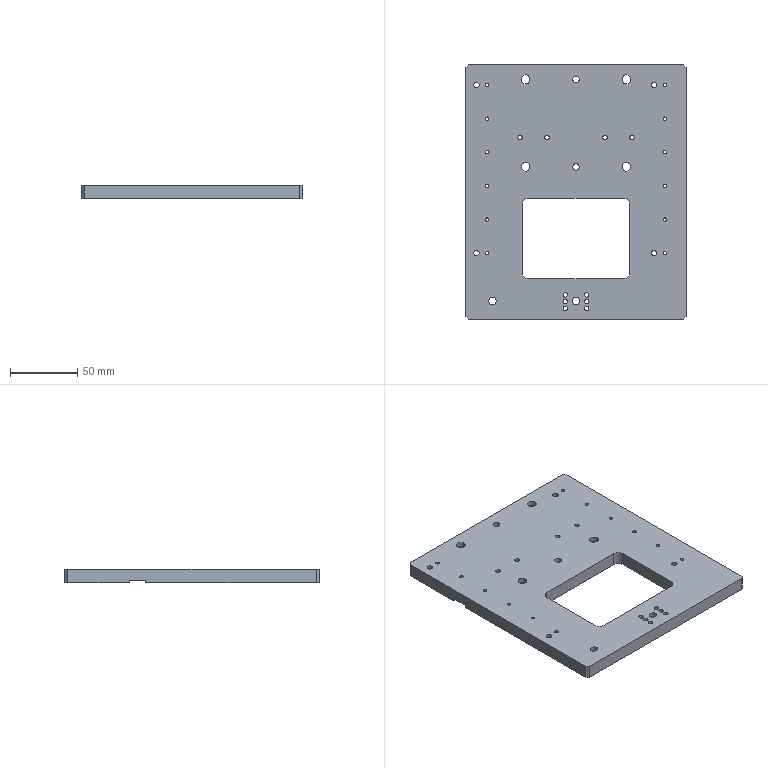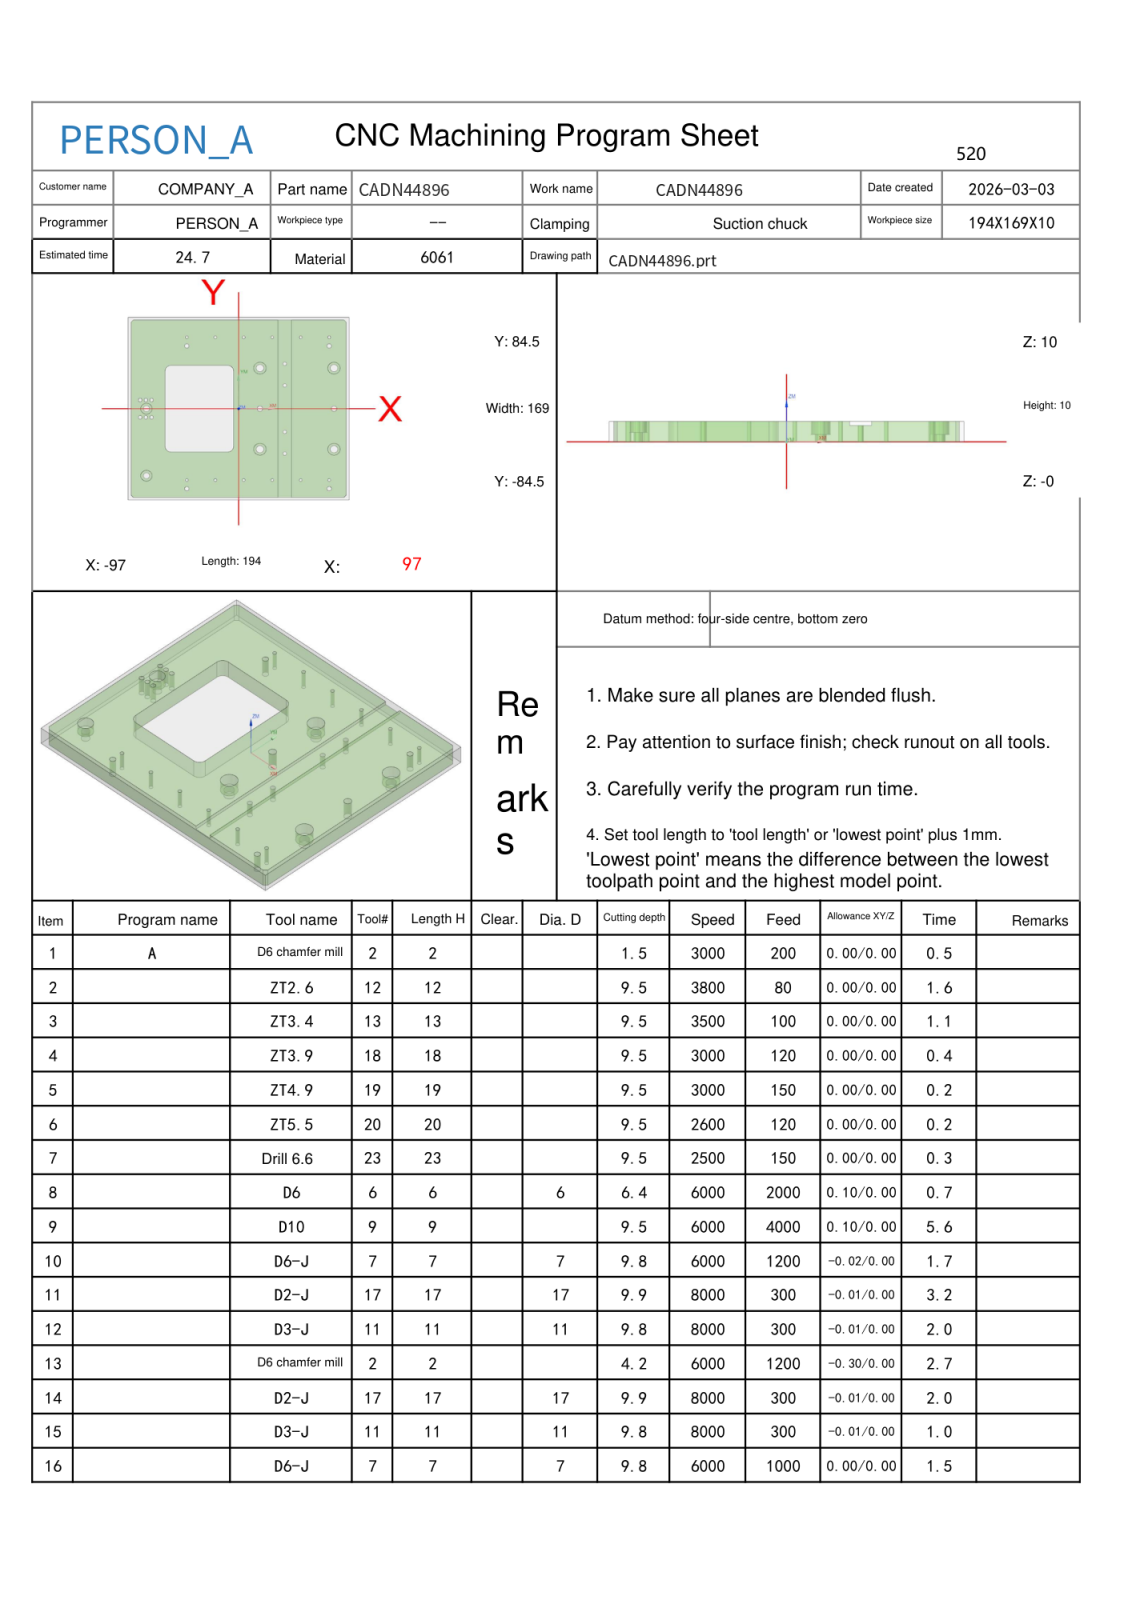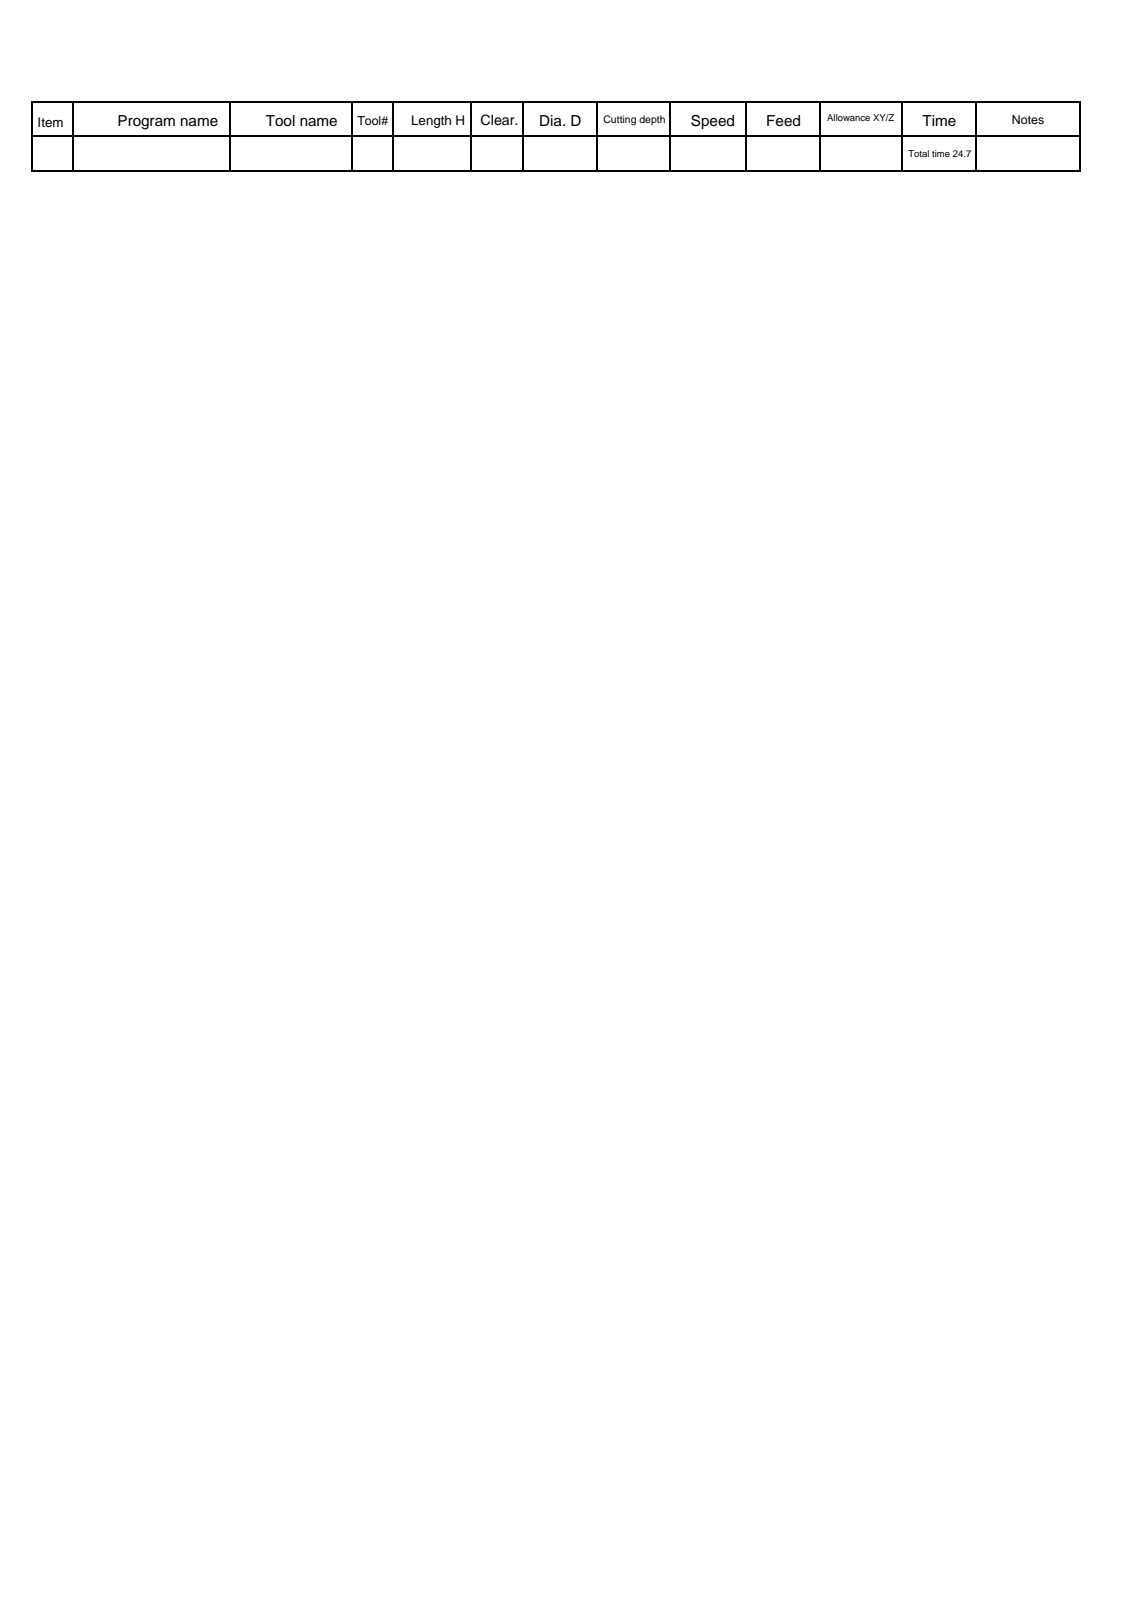NC program | NX | posted by the shop | part box 164 x 189 x 10 mm
Lines 2444 to 4061 of 4061, first 1295 of 1618 lines:
N12 T11 M06
(D3-J  D=3. R=0. H=11 ce=-0.01 di=0.00)
(D.N=11 MAX_Z=40. MIN_Z=0.15 Time=2.03M)
G00 G90 G54 X-81.065 Y1.225 M03 S8000
G43 H11 Z40.
M08
Z5.1
G01 X-81.111 Z5.098 F300.
X-81.384 Y1.169 Z5.083
X-81.637 Y1.053 Z5.068
X-81.857 Y.882 Z5.054
X-82.034 Y.667 Z5.039
X-82.157 Y.417 Z5.025
X-82.221 Y.146 Z5.01
X-82.225 Y-.111 Z4.997
X-82.167 Y-.389 Z4.982
X-82.046 Y-.647 Z4.967
X-81.87 Y-.87 Z4.952
X-81.647 Y-1.046 Z4.937
X-81.389 Y-1.167 Z4.922
X-81.111 Y-1.225 Z4.907
X-80.889 Z4.896
X-80.611 Y-1.167 Z4.881
X-80.353 Y-1.046 Z4.866
X-80.13 Y-.87 Z4.851
X-79.954 Y-.647 Z4.836
X-79.833 Y-.389 Z4.821
X-79.775 Y-.111 Z4.806
Y.111 Z4.794
X-79.833 Y.389 Z4.78
X-79.954 Y.647 Z4.765
X-80.13 Y.87 Z4.75
X-80.353 Y1.046 Z4.735
X-80.611 Y1.167 Z4.72
X-80.889 Y1.225 Z4.705
X-81.111 Z4.693
X-81.384 Y1.169 Z4.679
X-81.637 Y1.053 Z4.664
X-81.857 Y.882 Z4.65
X-82.034 Y.667 Z4.635
X-82.157 Y.417 Z4.62
X-82.221 Y.146 Z4.606
X-82.225 Y.035 Z4.6
G41 D11
X-82.26 Y0.0
G03 X-81. Y-1.26 Z4.476 I1.26 J0.0
X-79.74 Y0.0 Z4.353 I0.0 J1.26
X-81. Y1.26 Z4.229 I-1.26 J0.0
X-82.26 Y0.0 Z4.106 I0.0 J-1.26
X-81. Y-1.26 Z3.982 I1.26 J0.0
X-79.74 Y0.0 Z3.858 I0.0 J1.26
X-81. Y1.26 Z3.735 I-1.26 J0.0
X-82.26 Y0.0 Z3.611 I0.0 J-1.26
X-81. Y-1.26 Z3.488 I1.26 J0.0
X-79.74 Y0.0 Z3.364 I0.0 J1.26
X-81. Y1.26 Z3.24 I-1.26 J0.0
X-82.26 Y0.0 Z3.117 I0.0 J-1.26
X-81. Y-1.26 Z2.993 I1.26 J0.0
X-79.74 Y0.0 Z2.869 I0.0 J1.26
X-81. Y1.26 Z2.746 I-1.26 J0.0
X-82.26 Y0.0 Z2.622 I0.0 J-1.26
X-81. Y-1.26 Z2.499 I1.26 J0.0
X-79.74 Y0.0 Z2.375 I0.0 J1.26
X-81. Y1.26 Z2.251 I-1.26 J0.0
X-82.26 Y0.0 Z2.128 I0.0 J-1.26
X-81. Y-1.26 Z2.004 I1.26 J0.0
X-79.74 Y0.0 Z1.881 I0.0 J1.26
X-81. Y1.26 Z1.757 I-1.26 J0.0
X-82.26 Y0.0 Z1.633 I0.0 J-1.26
X-81. Y-1.26 Z1.51 I1.26 J0.0
X-79.74 Y0.0 Z1.386 I0.0 J1.26
X-81. Y1.26 Z1.263 I-1.26 J0.0
X-82.26 Y0.0 Z1.139 I0.0 J-1.26
X-81. Y-1.26 Z1.015 I1.26 J0.0
X-79.74 Y0.0 Z.892 I0.0 J1.26
X-81. Y1.26 Z.768 I-1.26 J0.0
X-82.26 Y0.0 Z.644 I0.0 J-1.26
X-81. Y-1.26 Z.521 I1.26 J0.0
X-79.74 Y0.0 Z.397 I0.0 J1.26
X-81. Y1.26 Z.274 I-1.26 J0.0
X-82.26 Y0.0 Z.15 I0.0 J-1.26
X-81. Y-1.26 I1.26 J0.0
X-79.74 Y0.0 I0.0 J1.26
X-81. Y1.26 I-1.26 J0.0
X-82.26 Y0.0 I0.0 J-1.26
X-82.197 Y-.393 I1.26 J0.0
G01 X-82.186 Y-.419
X-82.161 Y-.432
X-82.134 Y-.425
G40 X-82.086 Y-.41
Z1.15
G00 Z40.
X-81.065 Y-60.775
Z5.1
G01 X-81.111 Z5.098
X-81.384 Y-60.831 Z5.083
X-81.637 Y-60.947 Z5.068
X-81.857 Y-61.118 Z5.054
X-82.034 Y-61.333 Z5.039
X-82.157 Y-61.583 Z5.025
X-82.221 Y-61.854 Z5.01
X-82.225 Y-62.111 Z4.997
X-82.167 Y-62.389 Z4.982
X-82.046 Y-62.647 Z4.967
X-81.87 Y-62.87 Z4.952
X-81.647 Y-63.046 Z4.937
X-81.389 Y-63.167 Z4.922
X-81.111 Y-63.225 Z4.907
X-80.889 Z4.896
X-80.611 Y-63.167 Z4.881
X-80.353 Y-63.046 Z4.866
X-80.13 Y-62.87 Z4.851
X-79.954 Y-62.647 Z4.836
X-79.833 Y-62.389 Z4.821
X-79.775 Y-62.111 Z4.806
Y-61.889 Z4.794
X-79.833 Y-61.611 Z4.78
X-79.954 Y-61.353 Z4.765
X-80.13 Y-61.13 Z4.75
X-80.353 Y-60.954 Z4.735
X-80.611 Y-60.833 Z4.72
X-80.889 Y-60.775 Z4.705
X-81.111 Z4.693
X-81.384 Y-60.831 Z4.679
X-81.637 Y-60.947 Z4.664
X-81.857 Y-61.118 Z4.65
X-82.034 Y-61.333 Z4.635
X-82.157 Y-61.583 Z4.62
X-82.221 Y-61.854 Z4.606
X-82.225 Y-61.965 Z4.6
G41 D11
X-82.26 Y-62.
G03 X-81. Y-63.26 Z4.476 I1.26 J0.0
X-79.74 Y-62. Z4.353 I0.0 J1.26
X-81. Y-60.74 Z4.229 I-1.26 J0.0
X-82.26 Y-62. Z4.106 I0.0 J-1.26
X-81. Y-63.26 Z3.982 I1.26 J0.0
X-79.74 Y-62. Z3.858 I0.0 J1.26
X-81. Y-60.74 Z3.735 I-1.26 J0.0
X-82.26 Y-62. Z3.611 I0.0 J-1.26
X-81. Y-63.26 Z3.488 I1.26 J0.0
X-79.74 Y-62. Z3.364 I0.0 J1.26
X-81. Y-60.74 Z3.24 I-1.26 J0.0
X-82.26 Y-62. Z3.117 I0.0 J-1.26
X-81. Y-63.26 Z2.993 I1.26 J0.0
X-79.74 Y-62. Z2.869 I0.0 J1.26
X-81. Y-60.74 Z2.746 I-1.26 J0.0
X-82.26 Y-62. Z2.622 I0.0 J-1.26
X-81. Y-63.26 Z2.499 I1.26 J0.0
X-79.74 Y-62. Z2.375 I0.0 J1.26
X-81. Y-60.74 Z2.251 I-1.26 J0.0
X-82.26 Y-62. Z2.128 I0.0 J-1.26
X-81. Y-63.26 Z2.004 I1.26 J0.0
X-79.74 Y-62. Z1.881 I0.0 J1.26
X-81. Y-60.74 Z1.757 I-1.26 J0.0
X-82.26 Y-62. Z1.633 I0.0 J-1.26
X-81. Y-63.26 Z1.51 I1.26 J0.0
X-79.74 Y-62. Z1.386 I0.0 J1.26
X-81. Y-60.74 Z1.263 I-1.26 J0.0
X-82.26 Y-62. Z1.139 I0.0 J-1.26
X-81. Y-63.26 Z1.015 I1.26 J0.0
X-79.74 Y-62. Z.892 I0.0 J1.26
X-81. Y-60.74 Z.768 I-1.26 J0.0
X-82.26 Y-62. Z.644 I0.0 J-1.26
X-81. Y-63.26 Z.521 I1.26 J0.0
X-79.74 Y-62. Z.397 I0.0 J1.26
X-81. Y-60.74 Z.274 I-1.26 J0.0
X-82.26 Y-62. Z.15 I0.0 J-1.26
X-81. Y-63.26 I1.26 J0.0
X-79.74 Y-62. I0.0 J1.26
X-81. Y-60.74 I-1.26 J0.0
X-82.26 Y-62. I0.0 J-1.26
X-82.197 Y-62.393 I1.26 J0.0
G01 X-82.186 Y-62.419
X-82.161 Y-62.432
X-82.134 Y-62.425
G40 X-82.086 Y-62.41
Z1.15
G00 Z40.
X20.087 Y-38.613
Z4.1
G01 X20.278 Y-38.323 Z4.082
X20.412 Y-37.988 Z4.063
X20.475 Y-37.633 Z4.044
Y-37.367 Z4.03
X20.412 Y-37.012 Z4.011
X20.278 Y-36.677 Z3.992
X20.08 Y-36.375 Z3.973
X19.825 Y-36.12 Z3.954
X19.523 Y-35.922 Z3.936
X19.188 Y-35.788 Z3.917
X18.833 Y-35.725 Z3.898
X18.567 Z3.884
X18.212 Y-35.788 Z3.865
X17.877 Y-35.922 Z3.846
X17.575 Y-36.12 Z3.827
X17.32 Y-36.375 Z3.808
X17.122 Y-36.677 Z3.789
X16.988 Y-37.012 Z3.77
X16.925 Y-37.367 Z3.751
Y-37.633 Z3.737
X16.987 Y-37.984 Z3.719
X17.117 Y-38.314 Z3.7
X17.311 Y-38.613 Z3.682
X17.56 Y-38.867 Z3.663
X17.854 Y-39.066 Z3.644
X18.182 Y-39.203 Z3.626
X18.531 Y-39.272 Z3.607
X18.665 Y-39.275 Z3.6
G41 D11
X18.7 Y-39.31
G03 X20.51 Y-37.5 Z3.477 I0.0 J1.81
X18.7 Y-35.69 Z3.354 I-1.81 J0.0
X16.89 Y-37.5 Z3.23 I0.0 J-1.81
X18.7 Y-39.31 Z3.107 I1.81 J0.0
X20.51 Y-37.5 Z2.984 I0.0 J1.81
X18.7 Y-35.69 Z2.861 I-1.81 J0.0
X16.89 Y-37.5 Z2.738 I0.0 J-1.81
X18.7 Y-39.31 Z2.614 I1.81 J0.0
X20.51 Y-37.5 Z2.491 I0.0 J1.81
X18.7 Y-35.69 Z2.368 I-1.81 J0.0
X16.89 Y-37.5 Z2.245 I0.0 J-1.81
X18.7 Y-39.31 Z2.121 I1.81 J0.0
X20.51 Y-37.5 Z1.998 I0.0 J1.81
X18.7 Y-35.69 Z1.875 I-1.81 J0.0
X16.89 Y-37.5 Z1.752 I0.0 J-1.81
X18.7 Y-39.31 Z1.629 I1.81 J0.0
X20.51 Y-37.5 Z1.505 I0.0 J1.81
X18.7 Y-35.69 Z1.382 I-1.81 J0.0
X16.89 Y-37.5 Z1.259 I0.0 J-1.81
X18.7 Y-39.31 Z1.136 I1.81 J0.0
X20.51 Y-37.5 Z1.013 I0.0 J1.81
X18.7 Y-35.69 Z.889 I-1.81 J0.0
X16.89 Y-37.5 Z.766 I0.0 J-1.81
X18.7 Y-39.31 Z.643 I1.81 J0.0
X20.51 Y-37.5 Z.52 I0.0 J1.81
X18.7 Y-35.69 Z.396 I-1.81 J0.0
X16.89 Y-37.5 Z.273 I0.0 J-1.81
X18.7 Y-39.31 Z.15 I1.81 J0.0
X20.51 Y-37.5 I0.0 J1.81
X18.7 Y-35.69 I-1.81 J0.0
X16.89 Y-37.5 I0.0 J-1.81
X18.7 Y-39.31 I1.81 J0.0
X19.097 Y-39.266 I0.0 J1.81
G01 X19.123 Y-39.258
X19.138 Y-39.234
X19.135 Y-39.206
G40 X19.124 Y-39.157
Z1.15
G00 Z40.
X84.813 Y-36.112
Z4.1
G01 X84.523 Y-35.922 Z4.082
X84.188 Y-35.788 Z4.063
X83.833 Y-35.725 Z4.044
X83.567 Z4.03
X83.212 Y-35.788 Z4.011
X82.877 Y-35.922 Z3.992
X82.575 Y-36.12 Z3.973
X82.32 Y-36.375 Z3.954
X82.122 Y-36.677 Z3.936
X81.988 Y-37.012 Z3.917
X81.925 Y-37.367 Z3.898
Y-37.633 Z3.884
X81.963 Y-37.889 Z3.87
X82.037 Y-38.136 Z3.857
X82.147 Y-38.369 Z3.843
X82.294 Y-38.592 Z3.829
X82.551 Y-38.86 Z3.81
X82.858 Y-39.068 Z3.79
X83.201 Y-39.209 Z3.771
X83.567 Y-39.275 Z3.751
X83.833 Z3.737
X84.184 Y-39.213 Z3.719
X84.514 Y-39.083 Z3.7
X84.813 Y-38.889 Z3.682
X85.067 Y-38.64 Z3.663
X85.266 Y-38.346 Z3.644
X85.403 Y-38.018 Z3.626
X85.472 Y-37.669 Z3.607
X85.475 Y-37.535 Z3.6
G41 D11
X85.51 Y-37.5
G03 X83.7 Y-35.69 Z3.477 I-1.81 J0.0
X81.89 Y-37.5 Z3.354 I0.0 J-1.81
X82.191 Y-38.5 Z3.308 I1.81 J0.0
X83.7 Y-39.31 Z3.23 I1.509 J1.
X85.51 Y-37.5 Z3.107 I0.0 J1.81
X83.7 Y-35.69 Z2.984 I-1.81 J0.0
X81.89 Y-37.5 Z2.861 I0.0 J-1.81
X82.191 Y-38.5 Z2.815 I1.81 J0.0
X83.7 Y-39.31 Z2.738 I1.509 J1.
X85.51 Y-37.5 Z2.614 I0.0 J1.81
X83.7 Y-35.69 Z2.491 I-1.81 J0.0
X81.89 Y-37.5 Z2.368 I0.0 J-1.81
X82.191 Y-38.5 Z2.322 I1.81 J0.0
X83.7 Y-39.31 Z2.245 I1.509 J1.
X85.51 Y-37.5 Z2.121 I0.0 J1.81
X83.7 Y-35.69 Z1.998 I-1.81 J0.0
X81.89 Y-37.5 Z1.875 I0.0 J-1.81
X82.191 Y-38.5 Z1.829 I1.81 J0.0
X83.7 Y-39.31 Z1.752 I1.509 J1.
X85.51 Y-37.5 Z1.629 I0.0 J1.81
X83.7 Y-35.69 Z1.505 I-1.81 J0.0
X81.89 Y-37.5 Z1.382 I0.0 J-1.81
X82.191 Y-38.5 Z1.336 I1.81 J0.0
X83.7 Y-39.31 Z1.259 I1.509 J1.
X85.51 Y-37.5 Z1.136 I0.0 J1.81
X83.7 Y-35.69 Z1.013 I-1.81 J0.0
X81.89 Y-37.5 Z.889 I0.0 J-1.81
X82.191 Y-38.5 Z.843 I1.81 J0.0
X83.7 Y-39.31 Z.766 I1.509 J1.
X85.51 Y-37.5 Z.643 I0.0 J1.81
X83.7 Y-35.69 Z.52 I-1.81 J0.0
X81.89 Y-37.5 Z.396 I0.0 J-1.81
X82.191 Y-38.5 Z.351 I1.81 J0.0
X83.7 Y-39.31 Z.273 I1.509 J1.
X85.51 Y-37.5 Z.15 I0.0 J1.81
X83.7 Y-35.69 I-1.81 J0.0
X81.89 Y-37.5 I0.0 J-1.81
X83.7 Y-39.31 I1.81 J0.0
X85.51 Y-37.5 I0.0 J1.81
X85.466 Y-37.103 I-1.81 J0.0
G01 X85.458 Y-37.077
X85.434 Y-37.062
X85.406 Y-37.065
G40 X85.357 Y-37.076
Z1.15
G00 Z40.
X84.813 Y38.888
Z4.1
G01 X84.523 Y39.078 Z4.082
X84.188 Y39.212 Z4.063
X83.833 Y39.275 Z4.044
X83.567 Z4.03
X83.212 Y39.212 Z4.011
X82.877 Y39.078 Z3.992
X82.575 Y38.88 Z3.973
X82.32 Y38.625 Z3.954
X82.122 Y38.323 Z3.936
X81.988 Y37.988 Z3.917
X81.925 Y37.633 Z3.898
Y37.367 Z3.884
X81.963 Y37.111 Z3.87
X82.037 Y36.864 Z3.857
X82.147 Y36.631 Z3.843
X82.294 Y36.408 Z3.829
X82.551 Y36.14 Z3.81
X82.858 Y35.932 Z3.79
X83.201 Y35.791 Z3.771
X83.567 Y35.725 Z3.751
X83.833 Z3.737
X84.184 Y35.787 Z3.719
X84.514 Y35.917 Z3.7
X84.813 Y36.111 Z3.682
X85.067 Y36.36 Z3.663
X85.266 Y36.654 Z3.644
X85.403 Y36.982 Z3.626
X85.472 Y37.331 Z3.607
X85.475 Y37.465 Z3.6
G41 D11
X85.51 Y37.5
G03 X83.7 Y39.31 Z3.477 I-1.81 J0.0
X81.89 Y37.5 Z3.354 I0.0 J-1.81
X82.191 Y36.5 Z3.308 I1.81 J0.0
X83.7 Y35.69 Z3.23 I1.509 J1.
X85.51 Y37.5 Z3.107 I0.0 J1.81
X83.7 Y39.31 Z2.984 I-1.81 J0.0
X81.89 Y37.5 Z2.861 I0.0 J-1.81
X82.191 Y36.5 Z2.815 I1.81 J0.0
X83.7 Y35.69 Z2.738 I1.509 J1.
X85.51 Y37.5 Z2.614 I0.0 J1.81
X83.7 Y39.31 Z2.491 I-1.81 J0.0
X81.89 Y37.5 Z2.368 I0.0 J-1.81
X82.191 Y36.5 Z2.322 I1.81 J0.0
X83.7 Y35.69 Z2.245 I1.509 J1.
X85.51 Y37.5 Z2.121 I0.0 J1.81
X83.7 Y39.31 Z1.998 I-1.81 J0.0
X81.89 Y37.5 Z1.875 I0.0 J-1.81
X82.191 Y36.5 Z1.829 I1.81 J0.0
X83.7 Y35.69 Z1.752 I1.509 J1.
X85.51 Y37.5 Z1.629 I0.0 J1.81
X83.7 Y39.31 Z1.505 I-1.81 J0.0
X81.89 Y37.5 Z1.382 I0.0 J-1.81
X82.191 Y36.5 Z1.336 I1.81 J0.0
X83.7 Y35.69 Z1.259 I1.509 J1.
X85.51 Y37.5 Z1.136 I0.0 J1.81
X83.7 Y39.31 Z1.013 I-1.81 J0.0
X81.89 Y37.5 Z.889 I0.0 J-1.81
X82.191 Y36.5 Z.843 I1.81 J0.0
X83.7 Y35.69 Z.766 I1.509 J1.
X85.51 Y37.5 Z.643 I0.0 J1.81
X83.7 Y39.31 Z.52 I-1.81 J0.0
X81.89 Y37.5 Z.396 I0.0 J-1.81
X82.191 Y36.5 Z.351 I1.81 J0.0
X83.7 Y35.69 Z.273 I1.509 J1.
X85.51 Y37.5 Z.15 I0.0 J1.81
X83.7 Y39.31 I-1.81 J0.0
X81.89 Y37.5 I0.0 J-1.81
X83.7 Y35.69 I1.81 J0.0
X85.51 Y37.5 I0.0 J1.81
X85.466 Y37.897 I-1.81 J0.0
G01 X85.458 Y37.923
X85.434 Y37.938
X85.406 Y37.935
G40 X85.357 Y37.924
Z1.15
G00 Z40.
X17.313 Y38.613
Z4.1
G01 X17.122 Y38.323 Z4.082
X16.988 Y37.988 Z4.063
X16.925 Y37.633 Z4.044
Y37.367 Z4.03
X16.988 Y37.012 Z4.011
X17.122 Y36.677 Z3.992
X17.32 Y36.375 Z3.973
X17.575 Y36.12 Z3.954
X17.877 Y35.922 Z3.936
X18.212 Y35.788 Z3.917
X18.567 Y35.725 Z3.898
X18.833 Z3.884
X19.188 Y35.788 Z3.865
X19.523 Y35.922 Z3.846
X19.825 Y36.12 Z3.827
X20.08 Y36.375 Z3.808
X20.278 Y36.677 Z3.789
X20.412 Y37.012 Z3.77
X20.475 Y37.367 Z3.751
Y37.633 Z3.737
X20.413 Y37.984 Z3.719
X20.283 Y38.314 Z3.7
X20.089 Y38.613 Z3.682
X19.84 Y38.867 Z3.663
X19.546 Y39.066 Z3.644
X19.218 Y39.203 Z3.626
X18.869 Y39.272 Z3.607
X18.735 Y39.275 Z3.6
G41 D11
X18.7 Y39.31
G03 X16.89 Y37.5 Z3.477 I0.0 J-1.81
X18.7 Y35.69 Z3.354 I1.81 J0.0
X20.51 Y37.5 Z3.23 I0.0 J1.81
X18.7 Y39.31 Z3.107 I-1.81 J0.0
X16.89 Y37.5 Z2.984 I0.0 J-1.81
X18.7 Y35.69 Z2.861 I1.81 J0.0
X20.51 Y37.5 Z2.738 I0.0 J1.81
X18.7 Y39.31 Z2.614 I-1.81 J0.0
X16.89 Y37.5 Z2.491 I0.0 J-1.81
X18.7 Y35.69 Z2.368 I1.81 J0.0
X20.51 Y37.5 Z2.245 I0.0 J1.81
X18.7 Y39.31 Z2.121 I-1.81 J0.0
X16.89 Y37.5 Z1.998 I0.0 J-1.81
X18.7 Y35.69 Z1.875 I1.81 J0.0
X20.51 Y37.5 Z1.752 I0.0 J1.81
X18.7 Y39.31 Z1.629 I-1.81 J0.0
X16.89 Y37.5 Z1.505 I0.0 J-1.81
X18.7 Y35.69 Z1.382 I1.81 J0.0
X20.51 Y37.5 Z1.259 I0.0 J1.81
X18.7 Y39.31 Z1.136 I-1.81 J0.0
X16.89 Y37.5 Z1.013 I0.0 J-1.81
X18.7 Y35.69 Z.889 I1.81 J0.0
X20.51 Y37.5 Z.766 I0.0 J1.81
X18.7 Y39.31 Z.643 I-1.81 J0.0
X16.89 Y37.5 Z.52 I0.0 J-1.81
X18.7 Y35.69 Z.396 I1.81 J0.0
X20.51 Y37.5 Z.273 I0.0 J1.81
X18.7 Y39.31 Z.15 I-1.81 J0.0
X16.89 Y37.5 I0.0 J-1.81
X18.7 Y35.69 I1.81 J0.0
X20.51 Y37.5 I0.0 J1.81
X18.7 Y39.31 I-1.81 J0.0
X18.303 Y39.266 I0.0 J-1.81
G01 X18.277 Y39.258
X18.262 Y39.234
X18.265 Y39.206
G40 X18.276 Y39.157
Z1.15
G00 Z40.
G91 G28 Z0.0
M05
M09
G91 G28 Z0.0
M01
N13 T02 M06
(D6 chamfer mill  D=6. R=0. H=02 ce=0.00 di=0.00)
(MAX_Z=40. MIN_Z=5.8 Time=2.65M)
G00 G90 G54 X36.628 Y.25 M03 S6000
G43 H02 Z40.
M08
Z12.099
G01 Z8.5 F1200.
G03 X36.328 Y.33 I-.3 J-.52
X35.808 Y.03 I0.0 J-.6
G01 X35.8 Y0.0
Y-82.
G02 X34.5 Y-83.3 I-1.3 J0.0
G01 X-92.5
X-92.754 Y-83.275
X-92.997 Y-83.201
X-93.222 Y-83.081
X-93.419 Y-82.919
X-95.419 Y-80.919
X-95.581 Y-80.722
X-95.701 Y-80.497
X-95.775 Y-80.254
X-95.8 Y-80.
Y80.
X-95.775 Y80.254
X-95.701 Y80.497
X-95.581 Y80.722
X-95.419 Y80.919
X-93.419 Y82.919
X-93.222 Y83.081
X-92.997 Y83.201
X-92.754 Y83.275
X-92.5 Y83.3
X34.5
G02 X35.8 Y82. I0.0 J-1.3
G01 Y0.0
X35.808 Y-.03
G03 X36.328 Y-.33 I.52 J.3
X36.628 Y-.25 I0.0 J.6
G01 Z12.099
G00 Z40.
X-6.628
Z12.099
G01 Z8.5
G03 X-6.328 Y-.33 I.3 J.52
X-5.808 Y-.03 I0.0 J.6
G01 X-5.8 Y0.0
Y35.
G03 X-9.5 Y38.7 I-3.7 J0.0
G01 X-59.5
G03 X-63.2 Y35. I0.0 J-3.7
G01 Y-35.
G03 X-59.5 Y-38.7 I3.7 J0.0
G01 X-9.5
G03 X-5.8 Y-35. I0.0 J3.7
G01 Y0.0
X-5.808 Y.03
G03 X-6.328 Y.33 I-.52 J-.3
X-6.628 Y.25 I0.0 J-.6
G01 Z12.099
G00 Z40.
X44.372 Y-.25
Z12.099
G01 Z8.5
G03 X44.672 Y-.33 I.3 J.52
X45.192 Y-.03 I0.0 J.6
G01 X45.2 Y0.0
Y82.
G02 X46.5 Y83.3 I1.3 J0.0
G01 X92.5
X92.754 Y83.275
X92.997 Y83.201
X93.222 Y83.081
X93.419 Y82.919
X95.419 Y80.919
X95.581 Y80.722
X95.701 Y80.497
X95.775 Y80.254
X95.8 Y80.
Y-80.
X95.775 Y-80.254
X95.701 Y-80.497
X95.581 Y-80.722
X95.419 Y-80.919
X93.419 Y-82.919
X93.222 Y-83.081
X92.997 Y-83.201
X92.754 Y-83.275
X92.5 Y-83.3
X46.5
G02 X45.2 Y-82. I0.0 J1.3
G01 Y0.0
X45.192 Y.03
G03 X44.672 Y.33 I-.52 J-.3
X44.372 Y.25 I0.0 J-.6
G01 Z12.099
G00 Z40.
X43.468 Y-84.128
Z11.755
G01 Z6.501
G03 X43.549 Y-83.828 I-.52 J.3
X43.249 Y-83.308 I-.6 J0.0
G01 X43.219 Y-83.3
X37.781
X37.751 Y-83.308
G03 X37.451 Y-83.828 I.3 J-.52
X37.532 Y-84.128 I.6 J0.0
G01 Z11.755
G00 Z40.
Y84.128
Z11.755
G01 Z6.501
G03 X37.451 Y83.828 I.52 J-.3
X37.751 Y83.308 I.6 J0.0
G01 X37.781 Y83.3
X43.219
X43.249 Y83.308
G03 X43.549 Y83.828 I-.3 J.52
X43.468 Y84.128 I-.6 J0.0
G01 Z11.755
G00 Z40.
G00 G90 X79.5 Y-66. M03 S5000
Z40.
G98 G81 X79.5 Y-66. Z8.25 R13. F150.
X54.5
X29.5
X4.5
X-20.5
X-45.5
Y66.
X-20.5
X4.5
X29.5
X54.5
X79.5
G80
G00 Z40.
G00 G90 X-76.5 Y-8. M03 S5000
Z40.
G98 G81 X-76.5 Y-8. Z7.8 R13. F150.
X-81.5
X-86.5
Y8.
X-81.5
X-76.5
X40.5 Y41.5 Z5.8 R11.
Y21.5
Y-21.5
Y-41.5
G80
G00 Z40.
G00 G90 X-45.5 Y-74. M03 S5000
Z40.
G98 G81 X-45.5 Y-74. Z7.7 R13. F150.
X79.5
Y58.
X-45.5
G80
G00 Z40.
G00 G90 X83.7 Y0.0 M03 S5000
Z40.
G98 G81 X83.7 Y0.0 Z7.2 R13. F150.
X18.7
G80
G00 Z40.
G00 G90 X-78.711 Y.229 M03 S6000
Z40.
Z8.5
G01 Z8. F600.
X-78. Y.3
G03 X-81. Y3.3 I-3. J0.0
X-84.3 Y0.0 I0.0 J-3.3
X-81. Y-3.3 I3.3 J0.0
X-77.7 Y0.0 I0.0 J3.3
X-81. Y3.3 I-3.3 J0.0
X-84. Y.3 I0.0 J-3.
G01 X-83.289 Y.229
Z8.5
G00 Z40.
X-78.711 Y-61.771
Z8.5
G01 Z8.
X-78. Y-61.7
G03 X-81. Y-58.7 I-3. J0.0
X-84.3 Y-62. I0.0 J-3.3
X-81. Y-65.3 I3.3 J0.0
X-77.7 Y-62. I0.0 J3.3
X-81. Y-58.7 I-3.3 J0.0
X-84. Y-61.7 I0.0 J-3.
G01 X-83.289 Y-61.771
Z8.5
G00 Z40.
G00 G90 X86.405 Y38.221 M03 S6000
Z40.
Z8.5
G01 Z8. F600.
X86.7 Y38.3
G03 X83.7 Y41.3 I-3. J0.0
X79.9 Y37.5 I0.0 J-3.8
X83.7 Y33.7 I3.8 J0.0
X87.5 Y37.5 I0.0 J3.8
X83.7 Y41.3 I-3.8 J0.0
X80.7 Y38.3 I0.0 J-3.
G01 X80.995 Y38.221
Z8.5
G00 Z40.
X21.405
Z8.5
G01 Z8.
X21.7 Y38.3
G03 X18.7 Y41.3 I-3. J0.0
X14.9 Y37.5 I0.0 J-3.8
X18.7 Y33.7 I3.8 J0.0
X22.5 Y37.5 I0.0 J3.8
X18.7 Y41.3 I-3.8 J0.0
X15.7 Y38.3 I0.0 J-3.
G01 X15.995 Y38.221
Z8.5
G00 Z40.
X21.405 Y-36.779
Z8.5
G01 Z8.
X21.7 Y-36.7
G03 X18.7 Y-33.7 I-3. J0.0
X14.9 Y-37.5 I0.0 J-3.8
X18.7 Y-41.3 I3.8 J0.0
X22.5 Y-37.5 I0.0 J3.8
X18.7 Y-33.7 I-3.8 J0.0
X15.7 Y-36.7 I0.0 J-3.
G01 X15.995 Y-36.779
Z8.5
G00 Z40.
X86.405
Z8.5
G01 Z8.
X86.7 Y-36.7
G03 X83.7 Y-33.7 I-3. J0.0
X79.9 Y-37.5 I0.0 J-3.8
X83.7 Y-41.3 I3.8 J0.0
X87.5 Y-37.5 I0.0 J3.8
X83.7 Y-33.7 I-3.8 J0.0
X80.7 Y-36.7 I0.0 J-3.
G01 X80.995 Y-36.779
Z8.5
G00 Z40.
G91 G28 Z0.0
M05
M09
G91 G28 Z0.0
M01
N14 T17 M06
(D2-J  D=2. R=0. H=17 ce=-0.01 di=0.00)
(D.N=17 MAX_Z=40. MIN_Z=0.15 Time=1.98M)
G00 G90 G54 X-45.144 Y-73.087 M03 S8000
G43 H17 Z40.
M08
Z10.5
G01 X-45.401 Y-73.025 Z10.486 F300.
X-45.599 Z10.476
X-45.859 Y-73.088 Z10.462
X-46.092 Y-73.219 Z10.448
X-46.281 Y-73.408 Z10.434
X-46.412 Y-73.641 Z10.42
X-46.475 Y-73.901 Z10.406
Y-74.099 Z10.395
X-46.415 Y-74.352 Z10.382
X-46.29 Y-74.581 Z10.368
X-46.109 Y-74.768 Z10.354
X-45.885 Y-74.901 Z10.341
X-45.634 Y-74.971 Z10.327
X-45.401 Y-74.975 Z10.315
X-45.141 Y-74.912 Z10.301
X-44.908 Y-74.781 Z10.287
X-44.719 Y-74.592 Z10.273
X-44.588 Y-74.359 Z10.259
X-44.525 Y-74.099 Z10.245
Y-73.901 Z10.234
X-44.588 Y-73.641 Z10.22
X-44.719 Y-73.408 Z10.206
X-44.908 Y-73.219 Z10.192
X-45.141 Y-73.088 Z10.178
X-45.401 Y-73.025 Z10.164
X-45.599 Z10.154
X-45.859 Y-73.088 Z10.14
X-46.092 Y-73.219 Z10.126
X-46.281 Y-73.408 Z10.112
X-46.412 Y-73.641 Z10.098
X-46.475 Y-73.901 Z10.084
Y-74.099 Z10.073
X-46.415 Y-74.352 Z10.06
X-46.29 Y-74.581 Z10.046
X-46.109 Y-74.768 Z10.032
X-45.885 Y-74.901 Z10.019
X-45.634 Y-74.971 Z10.005
X-45.535 Y-74.975 Z10.
G41 D17
X-45.5 Y-75.01
G03 X-44.49 Y-74. Z9.877 I0.0 J1.01
X-45.5 Y-72.99 Z9.754 I-1.01 J0.0
X-46.51 Y-74. Z9.631 I0.0 J-1.01
X-45.5 Y-75.01 Z9.508 I1.01 J0.0
X-44.49 Y-74. Z9.384 I0.0 J1.01
X-45.5 Y-72.99 Z9.261 I-1.01 J0.0
X-46.51 Y-74. Z9.138 I0.0 J-1.01
X-45.5 Y-75.01 Z9.015 I1.01 J0.0
X-44.49 Y-74. Z8.892 I0.0 J1.01
X-45.5 Y-72.99 Z8.769 I-1.01 J0.0
X-46.51 Y-74. Z8.646 I0.0 J-1.01
X-45.5 Y-75.01 Z8.523 I1.01 J0.0
X-44.49 Y-74. Z8.399 I0.0 J1.01
X-45.5 Y-72.99 Z8.276 I-1.01 J0.0
X-46.51 Y-74. Z8.153 I0.0 J-1.01
X-45.5 Y-75.01 Z8.03 I1.01 J0.0
X-44.49 Y-74. Z7.907 I0.0 J1.01
X-45.5 Y-72.99 Z7.784 I-1.01 J0.0
X-46.51 Y-74. Z7.661 I0.0 J-1.01
X-45.5 Y-75.01 Z7.538 I1.01 J0.0
X-44.49 Y-74. Z7.414 I0.0 J1.01
X-45.5 Y-72.99 Z7.291 I-1.01 J0.0
X-46.51 Y-74. Z7.168 I0.0 J-1.01
X-45.5 Y-75.01 Z7.045 I1.01 J0.0
X-44.49 Y-74. Z6.922 I0.0 J1.01
X-45.5 Y-72.99 Z6.799 I-1.01 J0.0
X-46.51 Y-74. Z6.676 I0.0 J-1.01
X-45.5 Y-75.01 Z6.553 I1.01 J0.0
X-44.49 Y-74. Z6.429 I0.0 J1.01
X-45.5 Y-72.99 Z6.306 I-1.01 J0.0
X-46.51 Y-74. Z6.183 I0.0 J-1.01
X-45.5 Y-75.01 Z6.06 I1.01 J0.0
X-44.49 Y-74. Z5.937 I0.0 J1.01
X-45.5 Y-72.99 Z5.814 I-1.01 J0.0
X-46.51 Y-74. Z5.691 I0.0 J-1.01
X-45.5 Y-75.01 Z5.568 I1.01 J0.0
X-44.49 Y-74. Z5.444 I0.0 J1.01
X-45.5 Y-72.99 Z5.321 I-1.01 J0.0
X-46.51 Y-74. Z5.198 I0.0 J-1.01
X-45.5 Y-75.01 Z5.075 I1.01 J0.0
X-44.49 Y-74. Z4.952 I0.0 J1.01
X-45.5 Y-72.99 Z4.829 I-1.01 J0.0
X-46.51 Y-74. Z4.706 I0.0 J-1.01
X-45.5 Y-75.01 Z4.583 I1.01 J0.0
X-44.49 Y-74. Z4.459 I0.0 J1.01
X-45.5 Y-72.99 Z4.336 I-1.01 J0.0
X-46.51 Y-74. Z4.213 I0.0 J-1.01
X-45.5 Y-75.01 Z4.09 I1.01 J0.0
X-44.49 Y-74. Z3.967 I0.0 J1.01
X-45.5 Y-72.99 Z3.844 I-1.01 J0.0
X-46.51 Y-74. Z3.721 I0.0 J-1.01
X-45.5 Y-75.01 Z3.598 I1.01 J0.0
X-44.49 Y-74. Z3.474 I0.0 J1.01
X-45.5 Y-72.99 Z3.351 I-1.01 J0.0
X-46.51 Y-74. Z3.228 I0.0 J-1.01
X-45.5 Y-75.01 Z3.105 I1.01 J0.0
X-44.49 Y-74. Z2.982 I0.0 J1.01
X-45.5 Y-72.99 Z2.859 I-1.01 J0.0
X-46.51 Y-74. Z2.736 I0.0 J-1.01
X-45.5 Y-75.01 Z2.613 I1.01 J0.0
X-44.49 Y-74. Z2.489 I0.0 J1.01
X-45.5 Y-72.99 Z2.366 I-1.01 J0.0
X-46.51 Y-74. Z2.243 I0.0 J-1.01
X-45.5 Y-75.01 Z2.12 I1.01 J0.0
X-44.49 Y-74. Z1.997 I0.0 J1.01
X-45.5 Y-72.99 Z1.874 I-1.01 J0.0
X-46.51 Y-74. Z1.751 I0.0 J-1.01
X-45.5 Y-75.01 Z1.628 I1.01 J0.0
X-44.49 Y-74. Z1.504 I0.0 J1.01
X-45.5 Y-72.99 Z1.381 I-1.01 J0.0
X-46.51 Y-74. Z1.258 I0.0 J-1.01
X-45.5 Y-75.01 Z1.135 I1.01 J0.0
X-44.49 Y-74. Z1.012 I0.0 J1.01
X-45.5 Y-72.99 Z.889 I-1.01 J0.0
X-46.51 Y-74. Z.766 I0.0 J-1.01
X-45.5 Y-75.01 Z.643 I1.01 J0.0
X-44.49 Y-74. Z.519 I0.0 J1.01
X-45.5 Y-72.99 Z.396 I-1.01 J0.0
X-46.51 Y-74. Z.273 I0.0 J-1.01
X-45.5 Y-75.01 Z.15 I1.01 J0.0
X-44.49 Y-74. I0.0 J1.01
X-45.5 Y-72.99 I-1.01 J0.0
X-46.51 Y-74. I0.0 J-1.01
X-45.5 Y-75.01 I1.01 J0.0
X-45.11 Y-74.932 I0.0 J1.01
G01 X-45.086 Y-74.919
X-45.075 Y-74.893
X-45.084 Y-74.866
G40 X-45.103 Y-74.82
Z1.15
G00 Z40.
X79.856 Y-73.087
Z10.5
G01 X79.599 Y-73.025 Z10.486
X79.401 Z10.476
X79.141 Y-73.088 Z10.462
X78.908 Y-73.219 Z10.448
X78.719 Y-73.408 Z10.434
X78.588 Y-73.641 Z10.42
X78.525 Y-73.901 Z10.406
Y-74.099 Z10.395
X78.585 Y-74.352 Z10.382
X78.71 Y-74.581 Z10.368
X78.891 Y-74.768 Z10.354
X79.115 Y-74.901 Z10.341
X79.366 Y-74.971 Z10.327
X79.599 Y-74.975 Z10.315
X79.859 Y-74.912 Z10.301
X80.092 Y-74.781 Z10.287
X80.281 Y-74.592 Z10.273
X80.412 Y-74.359 Z10.259
X80.475 Y-74.099 Z10.245
Y-73.901 Z10.234
X80.412 Y-73.641 Z10.22
X80.281 Y-73.408 Z10.206
X80.092 Y-73.219 Z10.192
X79.859 Y-73.088 Z10.178
X79.599 Y-73.025 Z10.164
X79.401 Z10.154
X79.141 Y-73.088 Z10.14
X78.908 Y-73.219 Z10.126
X78.719 Y-73.408 Z10.112
X78.588 Y-73.641 Z10.098
X78.525 Y-73.901 Z10.084
Y-74.099 Z10.073
X78.585 Y-74.352 Z10.06
X78.71 Y-74.581 Z10.046
X78.891 Y-74.768 Z10.032
X79.115 Y-74.901 Z10.019
X79.366 Y-74.971 Z10.005
X79.465 Y-74.975 Z10.
G41 D17
X79.5 Y-75.01
G03 X80.51 Y-74. Z9.877 I0.0 J1.01
X79.5 Y-72.99 Z9.754 I-1.01 J0.0
X78.49 Y-74. Z9.631 I0.0 J-1.01
X79.5 Y-75.01 Z9.508 I1.01 J0.0
X80.51 Y-74. Z9.384 I0.0 J1.01
X79.5 Y-72.99 Z9.261 I-1.01 J0.0
X78.49 Y-74. Z9.138 I0.0 J-1.01
X79.5 Y-75.01 Z9.015 I1.01 J0.0
X80.51 Y-74. Z8.892 I0.0 J1.01
X79.5 Y-72.99 Z8.769 I-1.01 J0.0
X78.49 Y-74. Z8.646 I0.0 J-1.01
X79.5 Y-75.01 Z8.523 I1.01 J0.0
X80.51 Y-74. Z8.399 I0.0 J1.01
X79.5 Y-72.99 Z8.276 I-1.01 J0.0
X78.49 Y-74. Z8.153 I0.0 J-1.01
X79.5 Y-75.01 Z8.03 I1.01 J0.0
X80.51 Y-74. Z7.907 I0.0 J1.01
X79.5 Y-72.99 Z7.784 I-1.01 J0.0
X78.49 Y-74. Z7.661 I0.0 J-1.01
X79.5 Y-75.01 Z7.538 I1.01 J0.0
X80.51 Y-74. Z7.414 I0.0 J1.01
X79.5 Y-72.99 Z7.291 I-1.01 J0.0
X78.49 Y-74. Z7.168 I0.0 J-1.01
X79.5 Y-75.01 Z7.045 I1.01 J0.0
X80.51 Y-74. Z6.922 I0.0 J1.01
X79.5 Y-72.99 Z6.799 I-1.01 J0.0
X78.49 Y-74. Z6.676 I0.0 J-1.01
X79.5 Y-75.01 Z6.553 I1.01 J0.0
X80.51 Y-74. Z6.429 I0.0 J1.01
X79.5 Y-72.99 Z6.306 I-1.01 J0.0
X78.49 Y-74. Z6.183 I0.0 J-1.01
X79.5 Y-75.01 Z6.06 I1.01 J0.0
X80.51 Y-74. Z5.937 I0.0 J1.01
X79.5 Y-72.99 Z5.814 I-1.01 J0.0
X78.49 Y-74. Z5.691 I0.0 J-1.01
X79.5 Y-75.01 Z5.568 I1.01 J0.0
X80.51 Y-74. Z5.444 I0.0 J1.01
X79.5 Y-72.99 Z5.321 I-1.01 J0.0
X78.49 Y-74. Z5.198 I0.0 J-1.01
X79.5 Y-75.01 Z5.075 I1.01 J0.0
X80.51 Y-74. Z4.952 I0.0 J1.01
X79.5 Y-72.99 Z4.829 I-1.01 J0.0
X78.49 Y-74. Z4.706 I0.0 J-1.01
X79.5 Y-75.01 Z4.583 I1.01 J0.0
X80.51 Y-74. Z4.459 I0.0 J1.01
X79.5 Y-72.99 Z4.336 I-1.01 J0.0
X78.49 Y-74. Z4.213 I0.0 J-1.01
X79.5 Y-75.01 Z4.09 I1.01 J0.0
X80.51 Y-74. Z3.967 I0.0 J1.01
X79.5 Y-72.99 Z3.844 I-1.01 J0.0
X78.49 Y-74. Z3.721 I0.0 J-1.01
X79.5 Y-75.01 Z3.598 I1.01 J0.0
X80.51 Y-74. Z3.474 I0.0 J1.01
X79.5 Y-72.99 Z3.351 I-1.01 J0.0
X78.49 Y-74. Z3.228 I0.0 J-1.01
X79.5 Y-75.01 Z3.105 I1.01 J0.0
X80.51 Y-74. Z2.982 I0.0 J1.01
X79.5 Y-72.99 Z2.859 I-1.01 J0.0
X78.49 Y-74. Z2.736 I0.0 J-1.01
X79.5 Y-75.01 Z2.613 I1.01 J0.0
X80.51 Y-74. Z2.489 I0.0 J1.01
X79.5 Y-72.99 Z2.366 I-1.01 J0.0
X78.49 Y-74. Z2.243 I0.0 J-1.01
X79.5 Y-75.01 Z2.12 I1.01 J0.0
X80.51 Y-74. Z1.997 I0.0 J1.01
X79.5 Y-72.99 Z1.874 I-1.01 J0.0
X78.49 Y-74. Z1.751 I0.0 J-1.01
X79.5 Y-75.01 Z1.628 I1.01 J0.0
X80.51 Y-74. Z1.504 I0.0 J1.01
X79.5 Y-72.99 Z1.381 I-1.01 J0.0
X78.49 Y-74. Z1.258 I0.0 J-1.01
X79.5 Y-75.01 Z1.135 I1.01 J0.0
X80.51 Y-74. Z1.012 I0.0 J1.01
X79.5 Y-72.99 Z.889 I-1.01 J0.0
X78.49 Y-74. Z.766 I0.0 J-1.01
X79.5 Y-75.01 Z.643 I1.01 J0.0
X80.51 Y-74. Z.519 I0.0 J1.01
X79.5 Y-72.99 Z.396 I-1.01 J0.0
X78.49 Y-74. Z.273 I0.0 J-1.01
X79.5 Y-75.01 Z.15 I1.01 J0.0
X80.51 Y-74. I0.0 J1.01
X79.5 Y-72.99 I-1.01 J0.0
X78.49 Y-74. I0.0 J-1.01
X79.5 Y-75.01 I1.01 J0.0
X79.89 Y-74.932 I0.0 J1.01
G01 X79.914 Y-74.919
X79.925 Y-74.893
X79.916 Y-74.866
G40 X79.897 Y-74.82
Z1.15
G00 Z40.
X78.587 Y58.356
Z10.5
G01 X78.525 Y58.099 Z10.486
Y57.901 Z10.476
X78.588 Y57.641 Z10.462
X78.719 Y57.408 Z10.448
X78.908 Y57.219 Z10.434
X79.141 Y57.088 Z10.42
X79.401 Y57.025 Z10.406
X79.599 Z10.395
X79.852 Y57.085 Z10.382
X80.081 Y57.21 Z10.368
X80.268 Y57.391 Z10.354
X80.401 Y57.615 Z10.341
X80.471 Y57.866 Z10.327
X80.475 Y58.099 Z10.315
X80.412 Y58.359 Z10.301
X80.281 Y58.592 Z10.287
X80.092 Y58.781 Z10.273
X79.859 Y58.912 Z10.259
X79.599 Y58.975 Z10.245
X79.401 Z10.234
X79.141 Y58.912 Z10.22
X78.908 Y58.781 Z10.206
X78.719 Y58.592 Z10.192
X78.588 Y58.359 Z10.178
X78.525 Y58.099 Z10.164
Y57.901 Z10.154
X78.588 Y57.641 Z10.14
X78.719 Y57.408 Z10.126
X78.908 Y57.219 Z10.112
X79.141 Y57.088 Z10.098
X79.401 Y57.025 Z10.084
X79.599 Z10.073
X79.852 Y57.085 Z10.06
X80.081 Y57.21 Z10.046
X80.268 Y57.391 Z10.032
X80.401 Y57.615 Z10.019
X80.471 Y57.866 Z10.005
X80.475 Y57.965 Z10.
G41 D17
X80.51 Y58.
G03 X79.5 Y59.01 Z9.877 I-1.01 J0.0
X78.49 Y58. Z9.754 I0.0 J-1.01
X79.5 Y56.99 Z9.631 I1.01 J0.0
X80.51 Y58. Z9.508 I0.0 J1.01
X79.5 Y59.01 Z9.384 I-1.01 J0.0
X78.49 Y58. Z9.261 I0.0 J-1.01
X79.5 Y56.99 Z9.138 I1.01 J0.0
X80.51 Y58. Z9.015 I0.0 J1.01
X79.5 Y59.01 Z8.892 I-1.01 J0.0
X78.49 Y58. Z8.769 I0.0 J-1.01
X79.5 Y56.99 Z8.646 I1.01 J0.0
X80.51 Y58. Z8.523 I0.0 J1.01
X79.5 Y59.01 Z8.399 I-1.01 J0.0
X78.49 Y58. Z8.276 I0.0 J-1.01
X79.5 Y56.99 Z8.153 I1.01 J0.0
X80.51 Y58. Z8.03 I0.0 J1.01
X79.5 Y59.01 Z7.907 I-1.01 J0.0
X78.49 Y58. Z7.784 I0.0 J-1.01
X79.5 Y56.99 Z7.661 I1.01 J0.0
X80.51 Y58. Z7.538 I0.0 J1.01
X79.5 Y59.01 Z7.414 I-1.01 J0.0
X78.49 Y58. Z7.291 I0.0 J-1.01
X79.5 Y56.99 Z7.168 I1.01 J0.0
X80.51 Y58. Z7.045 I0.0 J1.01
X79.5 Y59.01 Z6.922 I-1.01 J0.0
X78.49 Y58. Z6.799 I0.0 J-1.01
X79.5 Y56.99 Z6.676 I1.01 J0.0
X80.51 Y58. Z6.553 I0.0 J1.01
X79.5 Y59.01 Z6.429 I-1.01 J0.0
X78.49 Y58. Z6.306 I0.0 J-1.01
X79.5 Y56.99 Z6.183 I1.01 J0.0
X80.51 Y58. Z6.06 I0.0 J1.01
X79.5 Y59.01 Z5.937 I-1.01 J0.0
X78.49 Y58. Z5.814 I0.0 J-1.01
X79.5 Y56.99 Z5.691 I1.01 J0.0
X80.51 Y58. Z5.568 I0.0 J1.01
X79.5 Y59.01 Z5.444 I-1.01 J0.0
X78.49 Y58. Z5.321 I0.0 J-1.01
X79.5 Y56.99 Z5.198 I1.01 J0.0
X80.51 Y58. Z5.075 I0.0 J1.01
X79.5 Y59.01 Z4.952 I-1.01 J0.0
X78.49 Y58. Z4.829 I0.0 J-1.01
X79.5 Y56.99 Z4.706 I1.01 J0.0
X80.51 Y58. Z4.583 I0.0 J1.01
X79.5 Y59.01 Z4.459 I-1.01 J0.0
X78.49 Y58. Z4.336 I0.0 J-1.01
X79.5 Y56.99 Z4.213 I1.01 J0.0
X80.51 Y58. Z4.09 I0.0 J1.01
X79.5 Y59.01 Z3.967 I-1.01 J0.0
X78.49 Y58. Z3.844 I0.0 J-1.01
X79.5 Y56.99 Z3.721 I1.01 J0.0
X80.51 Y58. Z3.598 I0.0 J1.01
X79.5 Y59.01 Z3.474 I-1.01 J0.0
X78.49 Y58. Z3.351 I0.0 J-1.01
X79.5 Y56.99 Z3.228 I1.01 J0.0
X80.51 Y58. Z3.105 I0.0 J1.01
X79.5 Y59.01 Z2.982 I-1.01 J0.0
X78.49 Y58. Z2.859 I0.0 J-1.01
X79.5 Y56.99 Z2.736 I1.01 J0.0
X80.51 Y58. Z2.613 I0.0 J1.01
X79.5 Y59.01 Z2.489 I-1.01 J0.0
X78.49 Y58. Z2.366 I0.0 J-1.01
X79.5 Y56.99 Z2.243 I1.01 J0.0
X80.51 Y58. Z2.12 I0.0 J1.01
X79.5 Y59.01 Z1.997 I-1.01 J0.0
X78.49 Y58. Z1.874 I0.0 J-1.01
X79.5 Y56.99 Z1.751 I1.01 J0.0
X80.51 Y58. Z1.628 I0.0 J1.01
X79.5 Y59.01 Z1.504 I-1.01 J0.0
X78.49 Y58. Z1.381 I0.0 J-1.01
X79.5 Y56.99 Z1.258 I1.01 J0.0
X80.51 Y58. Z1.135 I0.0 J1.01
X79.5 Y59.01 Z1.012 I-1.01 J0.0
X78.49 Y58. Z.889 I0.0 J-1.01
X79.5 Y56.99 Z.766 I1.01 J0.0
X80.51 Y58. Z.643 I0.0 J1.01
X79.5 Y59.01 Z.519 I-1.01 J0.0
X78.49 Y58. Z.396 I0.0 J-1.01
X79.5 Y56.99 Z.273 I1.01 J0.0
X80.51 Y58. Z.15 I0.0 J1.01
X79.5 Y59.01 I-1.01 J0.0
X78.49 Y58. I0.0 J-1.01
X79.5 Y56.99 I1.01 J0.0
X80.51 Y58. I0.0 J1.01
X80.432 Y58.39 I-1.01 J0.0
G01 X80.419 Y58.414
X80.393 Y58.425
X80.366 Y58.416
G40 X80.32 Y58.397
Z1.15
G00 Z40.
X-45.856 Y57.087
Z10.5
G01 X-45.599 Y57.025 Z10.486
X-45.401 Z10.476
X-45.141 Y57.088 Z10.462
X-44.908 Y57.219 Z10.448
X-44.719 Y57.408 Z10.434
X-44.588 Y57.641 Z10.42
X-44.525 Y57.901 Z10.406
Y58.099 Z10.395
X-44.585 Y58.352 Z10.382
X-44.71 Y58.581 Z10.368
X-44.891 Y58.768 Z10.354
X-45.115 Y58.901 Z10.341
X-45.366 Y58.971 Z10.327
X-45.599 Y58.975 Z10.315
X-45.859 Y58.912 Z10.301
X-46.092 Y58.781 Z10.287
X-46.281 Y58.592 Z10.273
X-46.412 Y58.359 Z10.259
X-46.475 Y58.099 Z10.245
Y57.901 Z10.234
X-46.412 Y57.641 Z10.22
X-46.281 Y57.408 Z10.206
X-46.092 Y57.219 Z10.192
X-45.859 Y57.088 Z10.178
X-45.599 Y57.025 Z10.164
X-45.401 Z10.154
X-45.141 Y57.088 Z10.14
X-44.908 Y57.219 Z10.126
X-44.719 Y57.408 Z10.112
X-44.588 Y57.641 Z10.098
X-44.525 Y57.901 Z10.084
Y58.099 Z10.073
X-44.585 Y58.352 Z10.06
X-44.71 Y58.581 Z10.046
X-44.891 Y58.768 Z10.032
X-45.115 Y58.901 Z10.019
X-45.366 Y58.971 Z10.005
X-45.465 Y58.975 Z10.
G41 D17
X-45.5 Y59.01
G03 X-46.51 Y58. Z9.877 I0.0 J-1.01
X-45.5 Y56.99 Z9.754 I1.01 J0.0
X-44.49 Y58. Z9.631 I0.0 J1.01
X-45.5 Y59.01 Z9.508 I-1.01 J0.0
X-46.51 Y58. Z9.384 I0.0 J-1.01
X-45.5 Y56.99 Z9.261 I1.01 J0.0
X-44.49 Y58. Z9.138 I0.0 J1.01
X-45.5 Y59.01 Z9.015 I-1.01 J0.0
X-46.51 Y58. Z8.892 I0.0 J-1.01
X-45.5 Y56.99 Z8.769 I1.01 J0.0
X-44.49 Y58. Z8.646 I0.0 J1.01
X-45.5 Y59.01 Z8.523 I-1.01 J0.0
X-46.51 Y58. Z8.399 I0.0 J-1.01
X-45.5 Y56.99 Z8.276 I1.01 J0.0
X-44.49 Y58. Z8.153 I0.0 J1.01
X-45.5 Y59.01 Z8.03 I-1.01 J0.0
X-46.51 Y58. Z7.907 I0.0 J-1.01
X-45.5 Y56.99 Z7.784 I1.01 J0.0
X-44.49 Y58. Z7.661 I0.0 J1.01
X-45.5 Y59.01 Z7.538 I-1.01 J0.0
X-46.51 Y58. Z7.414 I0.0 J-1.01
X-45.5 Y56.99 Z7.291 I1.01 J0.0
X-44.49 Y58. Z7.168 I0.0 J1.01
X-45.5 Y59.01 Z7.045 I-1.01 J0.0
X-46.51 Y58. Z6.922 I0.0 J-1.01
X-45.5 Y56.99 Z6.799 I1.01 J0.0
X-44.49 Y58. Z6.676 I0.0 J1.01
X-45.5 Y59.01 Z6.553 I-1.01 J0.0
X-46.51 Y58. Z6.429 I0.0 J-1.01
X-45.5 Y56.99 Z6.306 I1.01 J0.0
X-44.49 Y58. Z6.183 I0.0 J1.01
X-45.5 Y59.01 Z6.06 I-1.01 J0.0
X-46.51 Y58. Z5.937 I0.0 J-1.01
X-45.5 Y56.99 Z5.814 I1.01 J0.0
X-44.49 Y58. Z5.691 I0.0 J1.01
X-45.5 Y59.01 Z5.568 I-1.01 J0.0
X-46.51 Y58. Z5.444 I0.0 J-1.01
X-45.5 Y56.99 Z5.321 I1.01 J0.0
X-44.49 Y58. Z5.198 I0.0 J1.01
X-45.5 Y59.01 Z5.075 I-1.01 J0.0
X-46.51 Y58. Z4.952 I0.0 J-1.01
X-45.5 Y56.99 Z4.829 I1.01 J0.0
X-44.49 Y58. Z4.706 I0.0 J1.01
X-45.5 Y59.01 Z4.583 I-1.01 J0.0
X-46.51 Y58. Z4.459 I0.0 J-1.01
X-45.5 Y56.99 Z4.336 I1.01 J0.0
X-44.49 Y58. Z4.213 I0.0 J1.01
X-45.5 Y59.01 Z4.09 I-1.01 J0.0
X-46.51 Y58. Z3.967 I0.0 J-1.01
X-45.5 Y56.99 Z3.844 I1.01 J0.0
X-44.49 Y58. Z3.721 I0.0 J1.01
X-45.5 Y59.01 Z3.598 I-1.01 J0.0
X-46.51 Y58. Z3.474 I0.0 J-1.01
X-45.5 Y56.99 Z3.351 I1.01 J0.0
X-44.49 Y58. Z3.228 I0.0 J1.01
X-45.5 Y59.01 Z3.105 I-1.01 J0.0
X-46.51 Y58. Z2.982 I0.0 J-1.01
X-45.5 Y56.99 Z2.859 I1.01 J0.0
X-44.49 Y58. Z2.736 I0.0 J1.01
X-45.5 Y59.01 Z2.613 I-1.01 J0.0
X-46.51 Y58. Z2.489 I0.0 J-1.01
X-45.5 Y56.99 Z2.366 I1.01 J0.0
X-44.49 Y58. Z2.243 I0.0 J1.01
X-45.5 Y59.01 Z2.12 I-1.01 J0.0
X-46.51 Y58. Z1.997 I0.0 J-1.01
X-45.5 Y56.99 Z1.874 I1.01 J0.0
X-44.49 Y58. Z1.751 I0.0 J1.01
X-45.5 Y59.01 Z1.628 I-1.01 J0.0
X-46.51 Y58. Z1.504 I0.0 J-1.01
X-45.5 Y56.99 Z1.381 I1.01 J0.0
X-44.49 Y58. Z1.258 I0.0 J1.01
X-45.5 Y59.01 Z1.135 I-1.01 J0.0
X-46.51 Y58. Z1.012 I0.0 J-1.01
X-45.5 Y56.99 Z.889 I1.01 J0.0
X-44.49 Y58. Z.766 I0.0 J1.01
X-45.5 Y59.01 Z.643 I-1.01 J0.0
X-46.51 Y58. Z.519 I0.0 J-1.01
X-45.5 Y56.99 Z.396 I1.01 J0.0
X-44.49 Y58. Z.273 I0.0 J1.01
X-45.5 Y59.01 Z.15 I-1.01 J0.0
X-46.51 Y58. I0.0 J-1.01
X-45.5 Y56.99 I1.01 J0.0
X-44.49 Y58. I0.0 J1.01
X-45.5 Y59.01 I-1.01 J0.0
X-45.89 Y58.932 I0.0 J-1.01
G01 X-45.914 Y58.919
X-45.925 Y58.893
X-45.916 Y58.866
G40 X-45.897 Y58.82
Z1.15
G00 Z40.
G91 G28 Z0.0
M05
M09
G91 G28 Z0.0
M01
N15 T11 M06
(D3-J  D=3. R=0. H=11 ce=-0.01 di=0.00)
(D.N=11 MAX_Z=40. MIN_Z=0.15 Time=0.99M)
G00 G90 G54 X82.787 Y.356 M03 S8000
G43 H11 Z40.
M08
Z10.5
G01 X82.725 Y.099 Z10.486 F300.
Y-.099 Z10.476
X82.788 Y-.359 Z10.462
X82.919 Y-.592 Z10.448
X83.108 Y-.781 Z10.434
X83.341 Y-.912 Z10.42
X83.601 Y-.975 Z10.406
X83.799 Z10.395
X84.052 Y-.915 Z10.382
X84.281 Y-.79 Z10.368
X84.468 Y-.609 Z10.354
X84.601 Y-.385 Z10.341